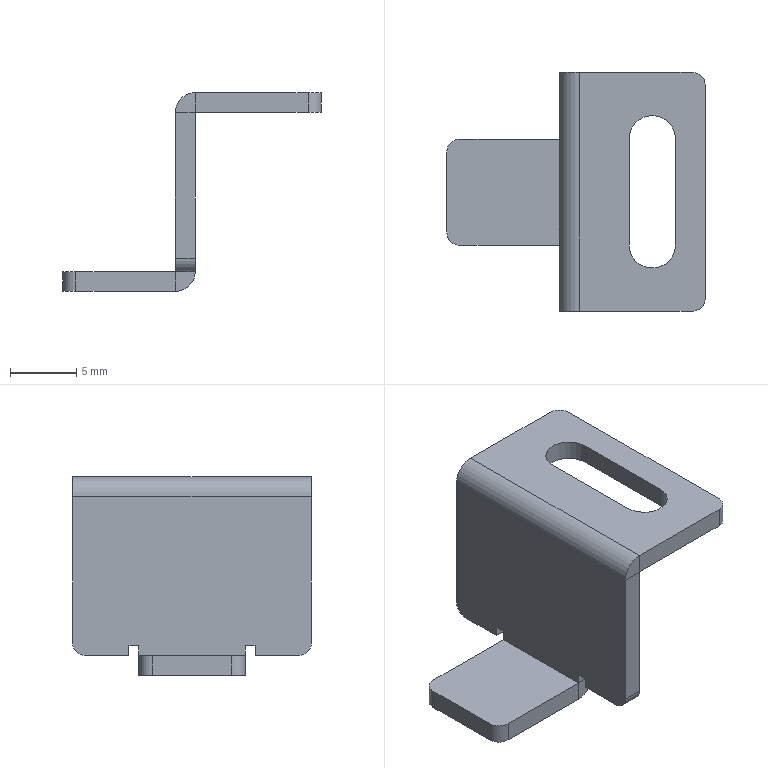Part | STEP file | 1 solid | 40 faces | box 19.5 x 18 x 15 mm | volume 668.205 mm3 | plane 28 | cylinder 12 | commonest cylinder face diameters 2 x6 0.02 x2 3.02 x2 3.5 x2